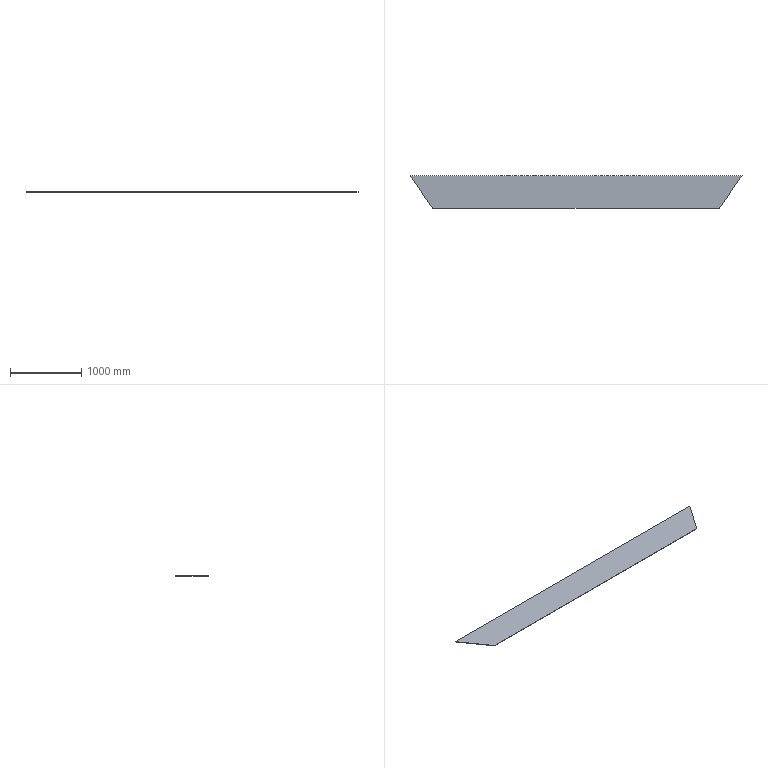Part | SolidWorks | features FlatPattern 1, SMBaseFlange 1, SheetMetal 1 | 1 solid | 6 faces | box 4660 x 455 x 5 mm | volume 9873500 mm3 | plane 6
STEP:
#1=CARTESIAN_POINT('',(0.,0.,0.));
#2=VERTEX_POINT('',#1);
#3=CARTESIAN_POINT('',(4020.,0.,0.));
#4=VERTEX_POINT('',#3);
#5=CARTESIAN_POINT('',(0.,0.,0.));
#6=DIRECTION('',(1.,0.,0.));
#7=VECTOR('',#6,1000.);
#8=LINE('',#5,#7);
#9=EDGE_CURVE('',#2,#4,#8,.T.);
#10=ORIENTED_EDGE('',*,*,#9,.F.);
#11=CARTESIAN_POINT('',(0.,0.,-5.));
#12=VERTEX_POINT('',#11);
#13=CARTESIAN_POINT('',(0.,0.,-5.));
#14=DIRECTION('',(0.,0.,1.));
#15=VECTOR('',#14,1000.);
#16=LINE('',#13,#15);
#17=EDGE_CURVE('',#12,#2,#16,.T.);
#18=ORIENTED_EDGE('',*,*,#17,.F.);
#19=CARTESIAN_POINT('',(4020.,0.,-5.));
#20=VERTEX_POINT('',#19);
#21=CARTESIAN_POINT('',(0.,0.,-5.));
#22=DIRECTION('',(1.,0.,0.));
#23=VECTOR('',#22,1000.);
#24=LINE('',#21,#23);
#25=EDGE_CURVE('',#12,#20,#24,.T.);
#26=ORIENTED_EDGE('',*,*,#25,.T.);
#27=CARTESIAN_POINT('',(4020.,0.,-5.));
#28=DIRECTION('',(0.,0.,1.));
#29=VECTOR('',#28,1000.);
#30=LINE('',#27,#29);
#31=EDGE_CURVE('',#20,#4,#30,.T.);
#32=ORIENTED_EDGE('',*,*,#31,.T.);
#33=EDGE_LOOP('',(#10,#18,#26,#32));
#34=FACE_OUTER_BOUND('',#33,.T.);
#35=CARTESIAN_POINT('',(0.,0.,-5.));
#36=DIRECTION('',(0.,-1.,0.));
#37=DIRECTION('',(0.,0.,-1.));
#38=AXIS2_PLACEMENT_3D('',#35,#36,#37);
#39=PLANE('',#38);
#40=ADVANCED_FACE('',(#34),#39,.T.);
#41=CARTESIAN_POINT('',(-320.,455.,0.));
#42=VERTEX_POINT('',#41);
#43=CARTESIAN_POINT('',(0.,0.,0.));
#44=DIRECTION('',(0.5753,-0.818,0.));
#45=VECTOR('',#44,1000.);
#46=LINE('',#43,#45);
#47=EDGE_CURVE('',#42,#2,#46,.T.);
#48=ORIENTED_EDGE('',*,*,#47,.F.);
#49=CARTESIAN_POINT('',(-320.,455.,-5.));
#50=VERTEX_POINT('',#49);
#51=CARTESIAN_POINT('',(-320.,455.,-5.));
#52=DIRECTION('',(0.,0.,1.));
#53=VECTOR('',#52,1000.);
#54=LINE('',#51,#53);
#55=EDGE_CURVE('',#50,#42,#54,.T.);
#56=ORIENTED_EDGE('',*,*,#55,.F.);
#57=CARTESIAN_POINT('',(0.,0.,-5.));
#58=DIRECTION('',(0.5753,-0.818,0.));
#59=VECTOR('',#58,1000.);
#60=LINE('',#57,#59);
#61=EDGE_CURVE('',#50,#12,#60,.T.);
#62=ORIENTED_EDGE('',*,*,#61,.T.);
#63=ORIENTED_EDGE('',*,*,#17,.T.);
#64=EDGE_LOOP('',(#48,#56,#62,#63));
#65=FACE_OUTER_BOUND('',#64,.T.);
#66=CARTESIAN_POINT('',(0.,0.,-5.));
#67=DIRECTION('',(-0.818,-0.5753,0.));
#68=DIRECTION('',(0.5753,-0.818,0.));
#69=AXIS2_PLACEMENT_3D('',#66,#67,#68);
#70=PLANE('',#69);
#71=ADVANCED_FACE('',(#65),#70,.T.);
#72=CARTESIAN_POINT('',(4340.,455.,0.));
#73=VERTEX_POINT('',#72);
#74=CARTESIAN_POINT('',(-320.,455.,0.));
#75=DIRECTION('',(-1.,0.,0.));
#76=VECTOR('',#75,1000.);
#77=LINE('',#74,#76);
#78=EDGE_CURVE('',#73,#42,#77,.T.);
#79=ORIENTED_EDGE('',*,*,#78,.F.);
#80=CARTESIAN_POINT('',(4340.,455.,-5.));
#81=VERTEX_POINT('',#80);
#82=CARTESIAN_POINT('',(4340.,455.,-5.));
#83=DIRECTION('',(0.,0.,1.));
#84=VECTOR('',#83,1000.);
#85=LINE('',#82,#84);
#86=EDGE_CURVE('',#81,#73,#85,.T.);
#87=ORIENTED_EDGE('',*,*,#86,.F.);
#88=CARTESIAN_POINT('',(-320.,455.,-5.));
#89=DIRECTION('',(-1.,0.,0.));
#90=VECTOR('',#89,1000.);
#91=LINE('',#88,#90);
#92=EDGE_CURVE('',#81,#50,#91,.T.);
#93=ORIENTED_EDGE('',*,*,#92,.T.);
#94=ORIENTED_EDGE('',*,*,#55,.T.);
#95=EDGE_LOOP('',(#79,#87,#93,#94));
#96=FACE_OUTER_BOUND('',#95,.T.);
#97=CARTESIAN_POINT('',(-320.,455.,-5.));
#98=DIRECTION('',(0.,1.,0.));
#99=DIRECTION('',(0.,0.,1.));
#100=AXIS2_PLACEMENT_3D('',#97,#98,#99);
#101=PLANE('',#100);
#102=ADVANCED_FACE('',(#96),#101,.T.);
#103=CARTESIAN_POINT('',(4020.,0.,0.));
#104=DIRECTION('',(0.5753,0.818,0.));
#105=VECTOR('',#104,1000.);
#106=LINE('',#103,#105);
#107=EDGE_CURVE('',#4,#73,#106,.T.);
#108=ORIENTED_EDGE('',*,*,#107,.F.);
#109=ORIENTED_EDGE('',*,*,#31,.F.);
#110=CARTESIAN_POINT('',(4020.,0.,-5.));
#111=DIRECTION('',(0.5753,0.818,0.));
#112=VECTOR('',#111,1000.);
#113=LINE('',#110,#112);
#114=EDGE_CURVE('',#20,#81,#113,.T.);
#115=ORIENTED_EDGE('',*,*,#114,.T.);
#116=ORIENTED_EDGE('',*,*,#86,.T.);
#117=EDGE_LOOP('',(#108,#109,#115,#116));
#118=FACE_OUTER_BOUND('',#117,.T.);
#119=CARTESIAN_POINT('',(4020.,0.,-5.));
#120=DIRECTION('',(0.818,-0.5753,0.));
#121=DIRECTION('',(0.5753,0.818,0.));
#122=AXIS2_PLACEMENT_3D('',#119,#120,#121);
#123=PLANE('',#122);
#124=ADVANCED_FACE('',(#118),#123,.T.);
#125=ORIENTED_EDGE('',*,*,#25,.F.);
#126=ORIENTED_EDGE('',*,*,#61,.F.);
#127=ORIENTED_EDGE('',*,*,#92,.F.);
#128=ORIENTED_EDGE('',*,*,#114,.F.);
#129=EDGE_LOOP('',(#125,#126,#127,#128));
#130=FACE_OUTER_BOUND('',#129,.T.);
#131=CARTESIAN_POINT('',(0.,0.,-5.));
#132=DIRECTION('',(0.,0.,1.));
#133=DIRECTION('',(1.,0.,0.));
#134=AXIS2_PLACEMENT_3D('',#131,#132,#133);
#135=PLANE('',#134);
#136=ADVANCED_FACE('',(#130),#135,.F.);
#137=ORIENTED_EDGE('',*,*,#9,.T.);
#138=ORIENTED_EDGE('',*,*,#107,.T.);
#139=ORIENTED_EDGE('',*,*,#78,.T.);
#140=ORIENTED_EDGE('',*,*,#47,.T.);
#141=EDGE_LOOP('',(#137,#138,#139,#140));
#142=FACE_OUTER_BOUND('',#141,.T.);
#143=CARTESIAN_POINT('',(0.,0.,0.));
#144=DIRECTION('',(0.,0.,1.));
#145=DIRECTION('',(1.,0.,0.));
#146=AXIS2_PLACEMENT_3D('',#143,#144,#145);
#147=PLANE('',#146);
#148=ADVANCED_FACE('',(#142),#147,.T.);
#149=CLOSED_SHELL('',(#40,#71,#102,#124,#136,#148));
#150=MANIFOLD_SOLID_BREP('',#149);
#151=CARTESIAN_POINT('',(0.,0.,0.));
#152=DIRECTION('',(0.,0.,1.));
#153=DIRECTION('',(1.,0.,0.));
#154=AXIS2_PLACEMENT_3D('',#151,#152,#153);
#155=(LENGTH_UNIT()NAMED_UNIT(*)SI_UNIT(.MILLI.,.METRE.));
#156=UNCERTAINTY_MEASURE_WITH_UNIT(LENGTH_MEASURE(0.00001),#155,'','');
#157=(NAMED_UNIT(*)PLANE_ANGLE_UNIT()SI_UNIT($,.RADIAN.));
#158=(NAMED_UNIT(*)SI_UNIT($,.STERADIAN.)SOLID_ANGLE_UNIT());
#159=(GEOMETRIC_REPRESENTATION_CONTEXT(3)GLOBAL_UNCERTAINTY_ASSIGNED_CONTEXT((#156))GLOBAL_UNIT_ASSIGNED_CONTEXT((#155,#157,#158))REPRESENTATION_CONTEXT('',''));
#160=ADVANCED_BREP_SHAPE_REPRESENTATION('',(#150,#154),#159);